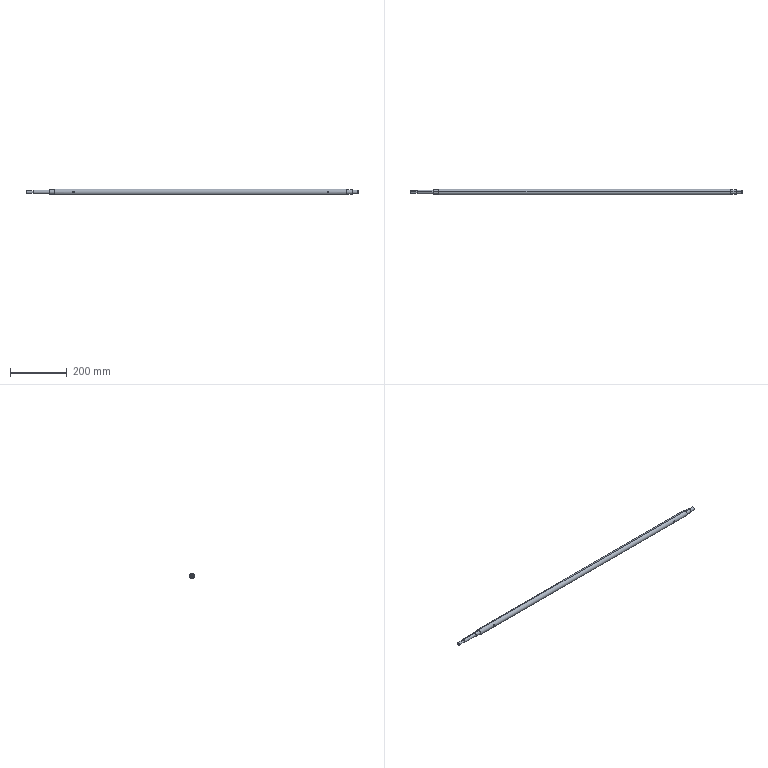Part | NX | features BREP 1 | 1 solid | 32 faces | box 1167 x 20 x 20 mm | volume 338692 mm3 | cylinder 18 | plane 10 | cone 4 | commonest cylinder face diameters 6 x4 12 x4 15 x4 4 x2 10 x2 20 x2
STEP:
#1=CARTESIAN_POINT('',(616.967,-9.539,-3.));
#2=VERTEX_POINT('',#1);
#3=CARTESIAN_POINT('',(616.967,-9.539,3.));
#4=VERTEX_POINT('',#3);
#5=CARTESIAN_POINT('',(616.967,-9.539,-3.));
#6=CARTESIAN_POINT('',(616.17,-9.539,-3.));
#7=CARTESIAN_POINT('',(614.623,-9.775,-2.35));
#8=CARTESIAN_POINT('',(613.639,-10.112,-0.004774));
#9=CARTESIAN_POINT('',(614.622,-9.775,2.351));
#10=CARTESIAN_POINT('',(616.17,-9.539,3.));
#11=CARTESIAN_POINT('',(616.967,-9.539,3.));
#12=B_SPLINE_CURVE_WITH_KNOTS('',3,(#5,#6,#7,#8,#9,#10,#11),.UNSPECIFIED.,.F.,.F.,(4,1,1,1,4),(0.,0.002358,0.004715,0.007073,0.009431),.UNSPECIFIED.);
#13=EDGE_CURVE('',#2,#4,#12,.T.);
#14=ORIENTED_EDGE('',*,*,#13,.F.);
#15=CARTESIAN_POINT('',(616.967,9.539,-3.));
#16=VERTEX_POINT('',#15);
#17=CARTESIAN_POINT('',(616.967,-10.,-3.));
#18=DIRECTION('',(0.,1.,0.));
#19=VECTOR('',#18,1000.);
#20=LINE('',#17,#19);
#21=EDGE_CURVE('',#2,#16,#20,.T.);
#22=ORIENTED_EDGE('',*,*,#21,.T.);
#23=CARTESIAN_POINT('',(616.967,9.539,3.));
#24=VERTEX_POINT('',#23);
#25=CARTESIAN_POINT('',(616.967,9.539,3.));
#26=CARTESIAN_POINT('',(616.17,9.539,3.));
#27=CARTESIAN_POINT('',(614.623,9.775,2.35));
#28=CARTESIAN_POINT('',(613.639,10.112,0.004774));
#29=CARTESIAN_POINT('',(614.622,9.775,-2.351));
#30=CARTESIAN_POINT('',(616.17,9.539,-3.));
#31=CARTESIAN_POINT('',(616.967,9.539,-3.));
#32=B_SPLINE_CURVE_WITH_KNOTS('',3,(#25,#26,#27,#28,#29,#30,#31),.UNSPECIFIED.,.F.,.F.,(4,1,1,1,4),(0.,0.002358,0.004715,0.007073,0.009431),.UNSPECIFIED.);
#33=EDGE_CURVE('',#24,#16,#32,.T.);
#34=ORIENTED_EDGE('',*,*,#33,.F.);
#35=CARTESIAN_POINT('',(616.967,-10.,3.));
#36=DIRECTION('',(0.,1.,0.));
#37=VECTOR('',#36,1000.);
#38=LINE('',#35,#37);
#39=EDGE_CURVE('',#4,#24,#38,.T.);
#40=ORIENTED_EDGE('',*,*,#39,.F.);
#41=EDGE_LOOP('',(#14,#22,#34,#40));
#42=FACE_BOUND('',#41,.T.);
#43=CARTESIAN_POINT('',(616.967,-10.,0.));
#44=DIRECTION('',(0.,1.,0.));
#45=DIRECTION('',(0.,0.,-1.));
#46=AXIS2_PLACEMENT_3D('',#43,#44,#45);
#47=CYLINDRICAL_SURFACE('',#46,3.);
#48=ADVANCED_FACE('',(#42),#47,.F.);
#49=CARTESIAN_POINT('',(-279.033,-9.539,-3.));
#50=VERTEX_POINT('',#49);
#51=CARTESIAN_POINT('',(-279.033,-9.539,3.));
#52=VERTEX_POINT('',#51);
#53=CARTESIAN_POINT('',(-279.033,-9.539,-3.));
#54=CARTESIAN_POINT('',(-279.83,-9.539,-3.));
#55=CARTESIAN_POINT('',(-281.377,-9.775,-2.35));
#56=CARTESIAN_POINT('',(-282.361,-10.112,-0.004774));
#57=CARTESIAN_POINT('',(-281.378,-9.775,2.351));
#58=CARTESIAN_POINT('',(-279.83,-9.539,3.));
#59=CARTESIAN_POINT('',(-279.033,-9.539,3.));
#60=B_SPLINE_CURVE_WITH_KNOTS('',3,(#53,#54,#55,#56,#57,#58,#59),.UNSPECIFIED.,.F.,.F.,(4,1,1,1,4),(0.,0.002358,0.004715,0.007073,0.009431),.UNSPECIFIED.);
#61=EDGE_CURVE('',#50,#52,#60,.T.);
#62=ORIENTED_EDGE('',*,*,#61,.F.);
#63=CARTESIAN_POINT('',(-279.033,9.539,-3.));
#64=VERTEX_POINT('',#63);
#65=CARTESIAN_POINT('',(-279.033,-10.,-3.));
#66=DIRECTION('',(0.,1.,0.));
#67=VECTOR('',#66,1000.);
#68=LINE('',#65,#67);
#69=EDGE_CURVE('',#50,#64,#68,.T.);
#70=ORIENTED_EDGE('',*,*,#69,.T.);
#71=CARTESIAN_POINT('',(-279.033,9.539,3.));
#72=VERTEX_POINT('',#71);
#73=CARTESIAN_POINT('',(-279.033,9.539,3.));
#74=CARTESIAN_POINT('',(-279.83,9.539,3.));
#75=CARTESIAN_POINT('',(-281.377,9.775,2.35));
#76=CARTESIAN_POINT('',(-282.361,10.112,0.004774));
#77=CARTESIAN_POINT('',(-281.378,9.775,-2.351));
#78=CARTESIAN_POINT('',(-279.83,9.539,-3.));
#79=CARTESIAN_POINT('',(-279.033,9.539,-3.));
#80=B_SPLINE_CURVE_WITH_KNOTS('',3,(#73,#74,#75,#76,#77,#78,#79),.UNSPECIFIED.,.F.,.F.,(4,1,1,1,4),(0.,0.002358,0.004715,0.007073,0.009431),.UNSPECIFIED.);
#81=EDGE_CURVE('',#72,#64,#80,.T.);
#82=ORIENTED_EDGE('',*,*,#81,.F.);
#83=CARTESIAN_POINT('',(-279.033,-10.,3.));
#84=DIRECTION('',(0.,1.,0.));
#85=VECTOR('',#84,1000.);
#86=LINE('',#83,#85);
#87=EDGE_CURVE('',#52,#72,#86,.T.);
#88=ORIENTED_EDGE('',*,*,#87,.F.);
#89=EDGE_LOOP('',(#62,#70,#82,#88));
#90=FACE_BOUND('',#89,.T.);
#91=CARTESIAN_POINT('',(-279.033,-10.,0.));
#92=DIRECTION('',(0.,1.,0.));
#93=DIRECTION('',(0.,0.,-1.));
#94=AXIS2_PLACEMENT_3D('',#91,#92,#93);
#95=CYLINDRICAL_SURFACE('',#94,3.);
#96=ADVANCED_FACE('',(#90),#95,.F.);
#97=CARTESIAN_POINT('',(721.967,0.,5.));
#98=VERTEX_POINT('',#97);
#99=CARTESIAN_POINT('',(721.967,0.,-5.));
#100=VERTEX_POINT('',#99);
#101=CARTESIAN_POINT('',(721.967,0.,0.));
#102=DIRECTION('',(-1.,0.,0.));
#103=DIRECTION('',(0.,0.,1.));
#104=AXIS2_PLACEMENT_3D('',#101,#102,#103);
#105=CIRCLE('',#104,5.);
#106=EDGE_CURVE('',#98,#100,#105,.T.);
#107=ORIENTED_EDGE('',*,*,#106,.T.);
#108=CARTESIAN_POINT('',(720.967,0.,-6.));
#109=VERTEX_POINT('',#108);
#110=CARTESIAN_POINT('',(721.967,0.,-5.));
#111=DIRECTION('',(-0.7071,0.,-0.7071));
#112=VECTOR('',#111,1000.);
#113=LINE('',#110,#112);
#114=EDGE_CURVE('',#100,#109,#113,.T.);
#115=ORIENTED_EDGE('',*,*,#114,.T.);
#116=CARTESIAN_POINT('',(720.967,0.,6.));
#117=VERTEX_POINT('',#116);
#118=CARTESIAN_POINT('',(720.967,0.,0.));
#119=DIRECTION('',(-1.,0.,0.));
#120=DIRECTION('',(0.,0.,1.));
#121=AXIS2_PLACEMENT_3D('',#118,#119,#120);
#122=CIRCLE('',#121,6.);
#123=EDGE_CURVE('',#117,#109,#122,.T.);
#124=ORIENTED_EDGE('',*,*,#123,.F.);
#125=CARTESIAN_POINT('',(721.967,0.,5.));
#126=DIRECTION('',(-0.7071,0.,0.7071));
#127=VECTOR('',#126,1000.);
#128=LINE('',#125,#127);
#129=EDGE_CURVE('',#98,#117,#128,.T.);
#130=ORIENTED_EDGE('',*,*,#129,.F.);
#131=EDGE_LOOP('',(#107,#115,#124,#130));
#132=FACE_BOUND('',#131,.T.);
#133=CARTESIAN_POINT('',(721.967,0.,0.));
#134=DIRECTION('',(-1.,0.,0.));
#135=DIRECTION('',(0.,0.,-1.));
#136=AXIS2_PLACEMENT_3D('',#133,#134,#135);
#137=CONICAL_SURFACE('',#136,5.,0.7854);
#138=ADVANCED_FACE('',(#132),#137,.T.);
#139=ORIENTED_EDGE('',*,*,#123,.T.);
#140=CARTESIAN_POINT('',(701.967,0.,-6.));
#141=VERTEX_POINT('',#140);
#142=CARTESIAN_POINT('',(-445.033,0.,-6.));
#143=DIRECTION('',(-1.,0.,0.));
#144=VECTOR('',#143,1000.);
#145=LINE('',#142,#144);
#146=EDGE_CURVE('',#109,#141,#145,.T.);
#147=ORIENTED_EDGE('',*,*,#146,.T.);
#148=CARTESIAN_POINT('',(701.967,0.,6.));
#149=VERTEX_POINT('',#148);
#150=CARTESIAN_POINT('',(701.967,0.,0.));
#151=DIRECTION('',(-1.,0.,0.));
#152=DIRECTION('',(0.,0.,1.));
#153=AXIS2_PLACEMENT_3D('',#150,#151,#152);
#154=CIRCLE('',#153,6.);
#155=EDGE_CURVE('',#149,#141,#154,.T.);
#156=ORIENTED_EDGE('',*,*,#155,.F.);
#157=CARTESIAN_POINT('',(-445.033,0.,6.));
#158=DIRECTION('',(-1.,0.,0.));
#159=VECTOR('',#158,1000.);
#160=LINE('',#157,#159);
#161=EDGE_CURVE('',#117,#149,#160,.T.);
#162=ORIENTED_EDGE('',*,*,#161,.F.);
#163=EDGE_LOOP('',(#139,#147,#156,#162));
#164=FACE_BOUND('',#163,.T.);
#165=CARTESIAN_POINT('',(-445.033,0.,0.));
#166=DIRECTION('',(-1.,0.,0.));
#167=DIRECTION('',(0.,0.,-1.));
#168=AXIS2_PLACEMENT_3D('',#165,#166,#167);
#169=CYLINDRICAL_SURFACE('',#168,6.);
#170=ADVANCED_FACE('',(#164),#169,.T.);
#171=CARTESIAN_POINT('',(701.967,0.,7.5));
#172=VERTEX_POINT('',#171);
#173=CARTESIAN_POINT('',(701.967,0.,-7.5));
#174=VERTEX_POINT('',#173);
#175=CARTESIAN_POINT('',(701.967,0.,0.));
#176=DIRECTION('',(-1.,0.,0.));
#177=DIRECTION('',(0.,0.,1.));
#178=AXIS2_PLACEMENT_3D('',#175,#176,#177);
#179=CIRCLE('',#178,7.5);
#180=EDGE_CURVE('',#172,#174,#179,.T.);
#181=ORIENTED_EDGE('',*,*,#180,.T.);
#182=CARTESIAN_POINT('',(681.967,0.,-7.5));
#183=VERTEX_POINT('',#182);
#184=CARTESIAN_POINT('',(-445.033,0.,-7.5));
#185=DIRECTION('',(-1.,0.,0.));
#186=VECTOR('',#185,1000.);
#187=LINE('',#184,#186);
#188=EDGE_CURVE('',#174,#183,#187,.T.);
#189=ORIENTED_EDGE('',*,*,#188,.T.);
#190=CARTESIAN_POINT('',(681.967,0.,7.5));
#191=VERTEX_POINT('',#190);
#192=CARTESIAN_POINT('',(681.967,0.,0.));
#193=DIRECTION('',(-1.,0.,0.));
#194=DIRECTION('',(0.,0.,1.));
#195=AXIS2_PLACEMENT_3D('',#192,#193,#194);
#196=CIRCLE('',#195,7.5);
#197=EDGE_CURVE('',#191,#183,#196,.T.);
#198=ORIENTED_EDGE('',*,*,#197,.F.);
#199=CARTESIAN_POINT('',(-445.033,0.,7.5));
#200=DIRECTION('',(-1.,0.,0.));
#201=VECTOR('',#200,1000.);
#202=LINE('',#199,#201);
#203=EDGE_CURVE('',#172,#191,#202,.T.);
#204=ORIENTED_EDGE('',*,*,#203,.F.);
#205=EDGE_LOOP('',(#181,#189,#198,#204));
#206=FACE_BOUND('',#205,.T.);
#207=CARTESIAN_POINT('',(-445.033,0.,0.));
#208=DIRECTION('',(-1.,0.,0.));
#209=DIRECTION('',(0.,0.,-1.));
#210=AXIS2_PLACEMENT_3D('',#207,#208,#209);
#211=CYLINDRICAL_SURFACE('',#210,7.5);
#212=ADVANCED_FACE('',(#206),#211,.T.);
#213=CARTESIAN_POINT('',(681.967,0.,10.));
#214=VERTEX_POINT('',#213);
#215=CARTESIAN_POINT('',(681.967,0.,-10.));
#216=VERTEX_POINT('',#215);
#217=CARTESIAN_POINT('',(681.967,0.,0.));
#218=DIRECTION('',(-1.,0.,0.));
#219=DIRECTION('',(0.,0.,1.));
#220=AXIS2_PLACEMENT_3D('',#217,#218,#219);
#221=CIRCLE('',#220,10.);
#222=EDGE_CURVE('',#214,#216,#221,.T.);
#223=ORIENTED_EDGE('',*,*,#222,.T.);
#224=CARTESIAN_POINT('',(-344.033,0.,-10.));
#225=VERTEX_POINT('',#224);
#226=CARTESIAN_POINT('',(-445.033,0.,-10.));
#227=DIRECTION('',(-1.,0.,0.));
#228=VECTOR('',#227,1000.);
#229=LINE('',#226,#228);
#230=EDGE_CURVE('',#216,#225,#229,.T.);
#231=ORIENTED_EDGE('',*,*,#230,.T.);
#232=CARTESIAN_POINT('',(-344.033,0.,10.));
#233=VERTEX_POINT('',#232);
#234=CARTESIAN_POINT('',(-344.033,0.,0.));
#235=DIRECTION('',(-1.,0.,0.));
#236=DIRECTION('',(0.,0.,1.));
#237=AXIS2_PLACEMENT_3D('',#234,#235,#236);
#238=CIRCLE('',#237,10.);
#239=EDGE_CURVE('',#233,#225,#238,.T.);
#240=ORIENTED_EDGE('',*,*,#239,.F.);
#241=CARTESIAN_POINT('',(-445.033,0.,10.));
#242=DIRECTION('',(-1.,0.,0.));
#243=VECTOR('',#242,1000.);
#244=LINE('',#241,#243);
#245=EDGE_CURVE('',#214,#233,#244,.T.);
#246=ORIENTED_EDGE('',*,*,#245,.F.);
#247=EDGE_LOOP('',(#223,#231,#240,#246));
#248=FACE_BOUND('',#247,.T.);
#249=ORIENTED_EDGE('',*,*,#81,.T.);
#250=CARTESIAN_POINT('',(-279.033,9.539,-3.));
#251=CARTESIAN_POINT('',(-278.235,9.539,-3.));
#252=CARTESIAN_POINT('',(-276.689,9.775,-2.35));
#253=CARTESIAN_POINT('',(-275.705,10.112,-0.004774));
#254=CARTESIAN_POINT('',(-276.688,9.775,2.351));
#255=CARTESIAN_POINT('',(-278.235,9.539,3.));
#256=CARTESIAN_POINT('',(-279.033,9.539,3.));
#257=B_SPLINE_CURVE_WITH_KNOTS('',3,(#250,#251,#252,#253,#254,#255,#256),.UNSPECIFIED.,.F.,.F.,(4,1,1,1,4),(0.,0.002358,0.004715,0.007073,0.009431),.UNSPECIFIED.);
#258=EDGE_CURVE('',#64,#72,#257,.T.);
#259=ORIENTED_EDGE('',*,*,#258,.T.);
#260=EDGE_LOOP('',(#249,#259));
#261=FACE_BOUND('',#260,.T.);
#262=ORIENTED_EDGE('',*,*,#33,.T.);
#263=CARTESIAN_POINT('',(616.967,9.539,-3.));
#264=CARTESIAN_POINT('',(617.765,9.539,-3.));
#265=CARTESIAN_POINT('',(619.311,9.775,-2.35));
#266=CARTESIAN_POINT('',(620.295,10.112,-0.004774));
#267=CARTESIAN_POINT('',(619.312,9.775,2.351));
#268=CARTESIAN_POINT('',(617.765,9.539,3.));
#269=CARTESIAN_POINT('',(616.967,9.539,3.));
#270=B_SPLINE_CURVE_WITH_KNOTS('',3,(#263,#264,#265,#266,#267,#268,#269),.UNSPECIFIED.,.F.,.F.,(4,1,1,1,4),(0.,0.002358,0.004715,0.007073,0.009431),.UNSPECIFIED.);
#271=EDGE_CURVE('',#16,#24,#270,.T.);
#272=ORIENTED_EDGE('',*,*,#271,.T.);
#273=EDGE_LOOP('',(#262,#272));
#274=FACE_BOUND('',#273,.T.);
#275=CARTESIAN_POINT('',(-445.033,0.,0.));
#276=DIRECTION('',(-1.,0.,0.));
#277=DIRECTION('',(0.,0.,-1.));
#278=AXIS2_PLACEMENT_3D('',#275,#276,#277);
#279=CYLINDRICAL_SURFACE('',#278,10.);
#280=ADVANCED_FACE('',(#248,#261,#274),#279,.T.);
#281=CARTESIAN_POINT('',(-344.033,0.,7.5));
#282=VERTEX_POINT('',#281);
#283=CARTESIAN_POINT('',(-344.033,0.,-7.5));
#284=VERTEX_POINT('',#283);
#285=CARTESIAN_POINT('',(-344.033,0.,0.));
#286=DIRECTION('',(-1.,0.,0.));
#287=DIRECTION('',(0.,0.,1.));
#288=AXIS2_PLACEMENT_3D('',#285,#286,#287);
#289=CIRCLE('',#288,7.5);
#290=EDGE_CURVE('',#282,#284,#289,.T.);
#291=ORIENTED_EDGE('',*,*,#290,.T.);
#292=CARTESIAN_POINT('',(-364.033,0.,-7.5));
#293=VERTEX_POINT('',#292);
#294=CARTESIAN_POINT('',(-445.033,0.,-7.5));
#295=DIRECTION('',(-1.,0.,0.));
#296=VECTOR('',#295,1000.);
#297=LINE('',#294,#296);
#298=EDGE_CURVE('',#284,#293,#297,.T.);
#299=ORIENTED_EDGE('',*,*,#298,.T.);
#300=CARTESIAN_POINT('',(-364.033,0.,7.5));
#301=VERTEX_POINT('',#300);
#302=CARTESIAN_POINT('',(-364.033,0.,0.));
#303=DIRECTION('',(-1.,0.,0.));
#304=DIRECTION('',(0.,0.,1.));
#305=AXIS2_PLACEMENT_3D('',#302,#303,#304);
#306=CIRCLE('',#305,7.5);
#307=EDGE_CURVE('',#301,#293,#306,.T.);
#308=ORIENTED_EDGE('',*,*,#307,.F.);
#309=CARTESIAN_POINT('',(-445.033,0.,7.5));
#310=DIRECTION('',(-1.,0.,0.));
#311=VECTOR('',#310,1000.);
#312=LINE('',#309,#311);
#313=EDGE_CURVE('',#282,#301,#312,.T.);
#314=ORIENTED_EDGE('',*,*,#313,.F.);
#315=EDGE_LOOP('',(#291,#299,#308,#314));
#316=FACE_BOUND('',#315,.T.);
#317=CARTESIAN_POINT('',(-445.033,0.,0.));
#318=DIRECTION('',(-1.,0.,0.));
#319=DIRECTION('',(0.,0.,-1.));
#320=AXIS2_PLACEMENT_3D('',#317,#318,#319);
#321=CYLINDRICAL_SURFACE('',#320,7.5);
#322=ADVANCED_FACE('',(#316),#321,.T.);
#323=CARTESIAN_POINT('',(-364.033,0.,6.));
#324=VERTEX_POINT('',#323);
#325=CARTESIAN_POINT('',(-364.033,0.,-6.));
#326=VERTEX_POINT('',#325);
#327=CARTESIAN_POINT('',(-364.033,0.,0.));
#328=DIRECTION('',(-1.,0.,0.));
#329=DIRECTION('',(0.,0.,1.));
#330=AXIS2_PLACEMENT_3D('',#327,#328,#329);
#331=CIRCLE('',#330,6.);
#332=EDGE_CURVE('',#324,#326,#331,.T.);
#333=ORIENTED_EDGE('',*,*,#332,.T.);
#334=CARTESIAN_POINT('',(-420.033,0.,-6.));
#335=VERTEX_POINT('',#334);
#336=CARTESIAN_POINT('',(-445.033,0.,-6.));
#337=DIRECTION('',(-1.,0.,0.));
#338=VECTOR('',#337,1000.);
#339=LINE('',#336,#338);
#340=EDGE_CURVE('',#326,#335,#339,.T.);
#341=ORIENTED_EDGE('',*,*,#340,.T.);
#342=CARTESIAN_POINT('',(-420.033,0.,6.));
#343=VERTEX_POINT('',#342);
#344=CARTESIAN_POINT('',(-420.033,0.,0.));
#345=DIRECTION('',(-1.,0.,0.));
#346=DIRECTION('',(0.,0.,1.));
#347=AXIS2_PLACEMENT_3D('',#344,#345,#346);
#348=CIRCLE('',#347,6.);
#349=EDGE_CURVE('',#343,#335,#348,.T.);
#350=ORIENTED_EDGE('',*,*,#349,.F.);
#351=CARTESIAN_POINT('',(-445.033,0.,6.));
#352=DIRECTION('',(-1.,0.,0.));
#353=VECTOR('',#352,1000.);
#354=LINE('',#351,#353);
#355=EDGE_CURVE('',#324,#343,#354,.T.);
#356=ORIENTED_EDGE('',*,*,#355,.F.);
#357=EDGE_LOOP('',(#333,#341,#350,#356));
#358=FACE_BOUND('',#357,.T.);
#359=CARTESIAN_POINT('',(-445.033,0.,0.));
#360=DIRECTION('',(-1.,0.,0.));
#361=DIRECTION('',(0.,0.,-1.));
#362=AXIS2_PLACEMENT_3D('',#359,#360,#361);
#363=CYLINDRICAL_SURFACE('',#362,6.);
#364=ADVANCED_FACE('',(#358),#363,.T.);
#365=CARTESIAN_POINT('',(-420.033,0.,5.));
#366=VERTEX_POINT('',#365);
#367=CARTESIAN_POINT('',(-420.033,0.,-5.));
#368=VERTEX_POINT('',#367);
#369=CARTESIAN_POINT('',(-420.033,0.,0.));
#370=DIRECTION('',(-1.,0.,0.));
#371=DIRECTION('',(0.,0.,1.));
#372=AXIS2_PLACEMENT_3D('',#369,#370,#371);
#373=CIRCLE('',#372,5.);
#374=EDGE_CURVE('',#366,#368,#373,.T.);
#375=ORIENTED_EDGE('',*,*,#374,.T.);
#376=CARTESIAN_POINT('',(-444.033,0.,-5.));
#377=VERTEX_POINT('',#376);
#378=CARTESIAN_POINT('',(-445.033,0.,-5.));
#379=DIRECTION('',(-1.,0.,0.));
#380=VECTOR('',#379,1000.);
#381=LINE('',#378,#380);
#382=EDGE_CURVE('',#368,#377,#381,.T.);
#383=ORIENTED_EDGE('',*,*,#382,.T.);
#384=CARTESIAN_POINT('',(-444.033,0.,5.));
#385=VERTEX_POINT('',#384);
#386=CARTESIAN_POINT('',(-444.033,0.,0.));
#387=DIRECTION('',(-1.,0.,0.));
#388=DIRECTION('',(0.,0.,1.));
#389=AXIS2_PLACEMENT_3D('',#386,#387,#388);
#390=CIRCLE('',#389,5.);
#391=EDGE_CURVE('',#385,#377,#390,.T.);
#392=ORIENTED_EDGE('',*,*,#391,.F.);
#393=CARTESIAN_POINT('',(-445.033,0.,5.));
#394=DIRECTION('',(-1.,0.,0.));
#395=VECTOR('',#394,1000.);
#396=LINE('',#393,#395);
#397=EDGE_CURVE('',#366,#385,#396,.T.);
#398=ORIENTED_EDGE('',*,*,#397,.F.);
#399=EDGE_LOOP('',(#375,#383,#392,#398));
#400=FACE_BOUND('',#399,.T.);
#401=CARTESIAN_POINT('',(-437.033,4.583,-2.));
#402=VERTEX_POINT('',#401);
#403=CARTESIAN_POINT('',(-425.033,4.583,-2.));
#404=VERTEX_POINT('',#403);
#405=CARTESIAN_POINT('',(-445.033,4.583,-2.));
#406=DIRECTION('',(1.,0.,0.));
#407=VECTOR('',#406,1000.);
#408=LINE('',#405,#407);
#409=EDGE_CURVE('',#402,#404,#408,.T.);
#410=ORIENTED_EDGE('',*,*,#409,.T.);
#411=CARTESIAN_POINT('',(-425.033,4.583,2.));
#412=VERTEX_POINT('',#411);
#413=CARTESIAN_POINT('',(-425.033,4.583,-2.));
#414=CARTESIAN_POINT('',(-424.498,4.583,-2.));
#415=CARTESIAN_POINT('',(-423.472,4.8,-1.567));
#416=CARTESIAN_POINT('',(-422.813,5.1,-0.004067));
#417=CARTESIAN_POINT('',(-423.472,4.8,1.568));
#418=CARTESIAN_POINT('',(-424.498,4.583,2.));
#419=CARTESIAN_POINT('',(-425.033,4.583,2.));
#420=B_SPLINE_CURVE_WITH_KNOTS('',3,(#413,#414,#415,#416,#417,#418,#419),.UNSPECIFIED.,.F.,.F.,(4,1,1,1,4),(0.,0.001579,0.003158,0.004737,0.006317),.UNSPECIFIED.);
#421=EDGE_CURVE('',#404,#412,#420,.T.);
#422=ORIENTED_EDGE('',*,*,#421,.T.);
#423=CARTESIAN_POINT('',(-437.033,4.583,2.));
#424=VERTEX_POINT('',#423);
#425=CARTESIAN_POINT('',(-445.033,4.583,2.));
#426=DIRECTION('',(-1.,0.,0.));
#427=VECTOR('',#426,1000.);
#428=LINE('',#425,#427);
#429=EDGE_CURVE('',#412,#424,#428,.T.);
#430=ORIENTED_EDGE('',*,*,#429,.T.);
#431=CARTESIAN_POINT('',(-437.033,4.583,2.));
#432=CARTESIAN_POINT('',(-437.567,4.583,2.));
#433=CARTESIAN_POINT('',(-438.593,4.8,1.567));
#434=CARTESIAN_POINT('',(-439.252,5.1,0.004067));
#435=CARTESIAN_POINT('',(-438.594,4.8,-1.568));
#436=CARTESIAN_POINT('',(-437.567,4.583,-2.));
#437=CARTESIAN_POINT('',(-437.033,4.583,-2.));
#438=B_SPLINE_CURVE_WITH_KNOTS('',3,(#431,#432,#433,#434,#435,#436,#437),.UNSPECIFIED.,.F.,.F.,(4,1,1,1,4),(0.,0.001579,0.003158,0.004737,0.006317),.UNSPECIFIED.);
#439=EDGE_CURVE('',#424,#402,#438,.T.);
#440=ORIENTED_EDGE('',*,*,#439,.T.);
#441=EDGE_LOOP('',(#410,#422,#430,#440));
#442=FACE_BOUND('',#441,.T.);
#443=CARTESIAN_POINT('',(-445.033,0.,0.));
#444=DIRECTION('',(-1.,0.,0.));
#445=DIRECTION('',(0.,0.,-1.));
#446=AXIS2_PLACEMENT_3D('',#443,#444,#445);
#447=CYLINDRICAL_SURFACE('',#446,5.);
#448=ADVANCED_FACE('',(#400,#442),#447,.T.);
#449=CARTESIAN_POINT('',(-445.033,0.,4.));
#450=VERTEX_POINT('',#449);
#451=CARTESIAN_POINT('',(-445.033,0.,-4.));
#452=VERTEX_POINT('',#451);
#453=CARTESIAN_POINT('',(-445.033,0.,0.));
#454=DIRECTION('',(-1.,0.,0.));
#455=DIRECTION('',(0.,0.,1.));
#456=AXIS2_PLACEMENT_3D('',#453,#454,#455);
#457=CIRCLE('',#456,4.);
#458=EDGE_CURVE('',#450,#452,#457,.T.);
#459=ORIENTED_EDGE('',*,*,#458,.F.);
#460=CARTESIAN_POINT('',(-444.033,0.,5.));
#461=DIRECTION('',(0.7071,0.,0.7071));
#462=VECTOR('',#461,1000.);
#463=LINE('',#460,#462);
#464=EDGE_CURVE('',#385,#450,#463,.F.);
#465=ORIENTED_EDGE('',*,*,#464,.F.);
#466=ORIENTED_EDGE('',*,*,#391,.T.);
#467=CARTESIAN_POINT('',(-444.033,0.,-5.));
#468=DIRECTION('',(0.7071,0.,-0.7071));
#469=VECTOR('',#468,1000.);
#470=LINE('',#467,#469);
#471=EDGE_CURVE('',#377,#452,#470,.F.);
#472=ORIENTED_EDGE('',*,*,#471,.T.);
#473=EDGE_LOOP('',(#459,#465,#466,#472));
#474=FACE_BOUND('',#473,.T.);
#475=CARTESIAN_POINT('',(-444.033,0.,0.));
#476=DIRECTION('',(1.,0.,0.));
#477=DIRECTION('',(0.,0.,1.));
#478=AXIS2_PLACEMENT_3D('',#475,#476,#477);
#479=CONICAL_SURFACE('',#478,5.,0.7854);
#480=ADVANCED_FACE('',(#474),#479,.T.);
#481=ORIENTED_EDGE('',*,*,#464,.T.);
#482=CARTESIAN_POINT('',(-445.033,0.,0.));
#483=DIRECTION('',(-1.,0.,0.));
#484=DIRECTION('',(0.,0.,1.));
#485=AXIS2_PLACEMENT_3D('',#482,#483,#484);
#486=CIRCLE('',#485,4.);
#487=EDGE_CURVE('',#452,#450,#486,.T.);
#488=ORIENTED_EDGE('',*,*,#487,.F.);
#489=ORIENTED_EDGE('',*,*,#471,.F.);
#490=CARTESIAN_POINT('',(-444.033,0.,0.));
#491=DIRECTION('',(-1.,0.,0.));
#492=DIRECTION('',(0.,0.,1.));
#493=AXIS2_PLACEMENT_3D('',#490,#491,#492);
#494=CIRCLE('',#493,5.);
#495=EDGE_CURVE('',#377,#385,#494,.T.);
#496=ORIENTED_EDGE('',*,*,#495,.T.);
#497=EDGE_LOOP('',(#481,#488,#489,#496));
#498=FACE_BOUND('',#497,.T.);
#499=CARTESIAN_POINT('',(-444.033,0.,0.));
#500=DIRECTION('',(1.,0.,0.));
#501=DIRECTION('',(0.,0.,1.));
#502=AXIS2_PLACEMENT_3D('',#499,#500,#501);
#503=CONICAL_SURFACE('',#502,5.,0.7854);
#504=ADVANCED_FACE('',(#498),#503,.T.);
#505=ORIENTED_EDGE('',*,*,#382,.F.);
#506=CARTESIAN_POINT('',(-420.033,0.,0.));
#507=DIRECTION('',(-1.,0.,0.));
#508=DIRECTION('',(0.,0.,1.));
#509=AXIS2_PLACEMENT_3D('',#506,#507,#508);
#510=CIRCLE('',#509,5.);
#511=EDGE_CURVE('',#368,#366,#510,.T.);
#512=ORIENTED_EDGE('',*,*,#511,.T.);
#513=ORIENTED_EDGE('',*,*,#397,.T.);
#514=ORIENTED_EDGE('',*,*,#495,.F.);
#515=EDGE_LOOP('',(#505,#512,#513,#514));
#516=FACE_BOUND('',#515,.T.);
#517=CARTESIAN_POINT('',(-445.033,0.,0.));
#518=DIRECTION('',(-1.,0.,0.));
#519=DIRECTION('',(0.,0.,-1.));
#520=AXIS2_PLACEMENT_3D('',#517,#518,#519);
#521=CYLINDRICAL_SURFACE('',#520,5.);
#522=ADVANCED_FACE('',(#516),#521,.T.);
#523=ORIENTED_EDGE('',*,*,#349,.T.);
#524=CARTESIAN_POINT('',(-420.033,0.,0.));
#525=DIRECTION('',(-1.,0.,0.));
#526=DIRECTION('',(0.,0.,1.));
#527=AXIS2_PLACEMENT_3D('',#524,#525,#526);
#528=CIRCLE('',#527,6.);
#529=EDGE_CURVE('',#335,#343,#528,.T.);
#530=ORIENTED_EDGE('',*,*,#529,.T.);
#531=EDGE_LOOP('',(#523,#530));
#532=FACE_BOUND('',#531,.T.);
#533=ORIENTED_EDGE('',*,*,#374,.F.);
#534=ORIENTED_EDGE('',*,*,#511,.F.);
#535=EDGE_LOOP('',(#533,#534));
#536=FACE_BOUND('',#535,.T.);
#537=CARTESIAN_POINT('',(-420.033,5.,0.));
#538=DIRECTION('',(1.,0.,0.));
#539=DIRECTION('',(0.,0.,1.));
#540=AXIS2_PLACEMENT_3D('',#537,#538,#539);
#541=PLANE('',#540);
#542=ADVANCED_FACE('',(#532,#536),#541,.F.);
#543=ORIENTED_EDGE('',*,*,#340,.F.);
#544=CARTESIAN_POINT('',(-364.033,0.,0.));
#545=DIRECTION('',(-1.,0.,0.));
#546=DIRECTION('',(0.,0.,1.));
#547=AXIS2_PLACEMENT_3D('',#544,#545,#546);
#548=CIRCLE('',#547,6.);
#549=EDGE_CURVE('',#326,#324,#548,.T.);
#550=ORIENTED_EDGE('',*,*,#549,.T.);
#551=ORIENTED_EDGE('',*,*,#355,.T.);
#552=ORIENTED_EDGE('',*,*,#529,.F.);
#553=EDGE_LOOP('',(#543,#550,#551,#552));
#554=FACE_BOUND('',#553,.T.);
#555=CARTESIAN_POINT('',(-445.033,0.,0.));
#556=DIRECTION('',(-1.,0.,0.));
#557=DIRECTION('',(0.,0.,-1.));
#558=AXIS2_PLACEMENT_3D('',#555,#556,#557);
#559=CYLINDRICAL_SURFACE('',#558,6.);
#560=ADVANCED_FACE('',(#554),#559,.T.);
#561=ORIENTED_EDGE('',*,*,#307,.T.);
#562=CARTESIAN_POINT('',(-364.033,0.,0.));
#563=DIRECTION('',(-1.,0.,0.));
#564=DIRECTION('',(0.,0.,1.));
#565=AXIS2_PLACEMENT_3D('',#562,#563,#564);
#566=CIRCLE('',#565,7.5);
#567=EDGE_CURVE('',#293,#301,#566,.T.);
#568=ORIENTED_EDGE('',*,*,#567,.T.);
#569=EDGE_LOOP('',(#561,#568));
#570=FACE_BOUND('',#569,.T.);
#571=ORIENTED_EDGE('',*,*,#332,.F.);
#572=ORIENTED_EDGE('',*,*,#549,.F.);
#573=EDGE_LOOP('',(#571,#572));
#574=FACE_BOUND('',#573,.T.);
#575=CARTESIAN_POINT('',(-364.033,6.,0.));
#576=DIRECTION('',(1.,0.,0.));
#577=DIRECTION('',(0.,0.,1.));
#578=AXIS2_PLACEMENT_3D('',#575,#576,#577);
#579=PLANE('',#578);
#580=ADVANCED_FACE('',(#570,#574),#579,.F.);
#581=ORIENTED_EDGE('',*,*,#298,.F.);
#582=CARTESIAN_POINT('',(-344.033,0.,0.));
#583=DIRECTION('',(-1.,0.,0.));
#584=DIRECTION('',(0.,0.,1.));
#585=AXIS2_PLACEMENT_3D('',#582,#583,#584);
#586=CIRCLE('',#585,7.5);
#587=EDGE_CURVE('',#284,#282,#586,.T.);
#588=ORIENTED_EDGE('',*,*,#587,.T.);
#589=ORIENTED_EDGE('',*,*,#313,.T.);
#590=ORIENTED_EDGE('',*,*,#567,.F.);
#591=EDGE_LOOP('',(#581,#588,#589,#590));
#592=FACE_BOUND('',#591,.T.);
#593=CARTESIAN_POINT('',(-445.033,0.,0.));
#594=DIRECTION('',(-1.,0.,0.));
#595=DIRECTION('',(0.,0.,-1.));
#596=AXIS2_PLACEMENT_3D('',#593,#594,#595);
#597=CYLINDRICAL_SURFACE('',#596,7.5);
#598=ADVANCED_FACE('',(#592),#597,.T.);
#599=ORIENTED_EDGE('',*,*,#239,.T.);
#600=CARTESIAN_POINT('',(-344.033,0.,0.));
#601=DIRECTION('',(-1.,0.,0.));
#602=DIRECTION('',(0.,0.,1.));
#603=AXIS2_PLACEMENT_3D('',#600,#601,#602);
#604=CIRCLE('',#603,10.);
#605=EDGE_CURVE('',#225,#233,#604,.T.);
#606=ORIENTED_EDGE('',*,*,#605,.T.);
#607=EDGE_LOOP('',(#599,#606));
#608=FACE_BOUND('',#607,.T.);
#609=ORIENTED_EDGE('',*,*,#290,.F.);
#610=ORIENTED_EDGE('',*,*,#587,.F.);
#611=EDGE_LOOP('',(#609,#610));
#612=FACE_BOUND('',#611,.T.);
#613=CARTESIAN_POINT('',(-344.033,7.5,0.));
#614=DIRECTION('',(1.,0.,0.));
#615=DIRECTION('',(0.,0.,1.));
#616=AXIS2_PLACEMENT_3D('',#613,#614,#615);
#617=PLANE('',#616);
#618=ADVANCED_FACE('',(#608,#612),#617,.F.);
#619=ORIENTED_EDGE('',*,*,#230,.F.);
#620=CARTESIAN_POINT('',(681.967,0.,0.));
#621=DIRECTION('',(-1.,0.,0.));
#622=DIRECTION('',(0.,0.,1.));
#623=AXIS2_PLACEMENT_3D('',#620,#621,#622);
#624=CIRCLE('',#623,10.);
#625=EDGE_CURVE('',#216,#214,#624,.T.);
#626=ORIENTED_EDGE('',*,*,#625,.T.);
#627=ORIENTED_EDGE('',*,*,#245,.T.);
#628=ORIENTED_EDGE('',*,*,#605,.F.);
#629=EDGE_LOOP('',(#619,#626,#627,#628));
#630=FACE_BOUND('',#629,.T.);
#631=CARTESIAN_POINT('',(616.967,-9.539,3.));
#632=CARTESIAN_POINT('',(617.765,-9.539,3.));
#633=CARTESIAN_POINT('',(619.311,-9.775,2.35));
#634=CARTESIAN_POINT('',(620.295,-10.112,0.004774));
#635=CARTESIAN_POINT('',(619.312,-9.775,-2.351));
#636=CARTESIAN_POINT('',(617.765,-9.539,-3.));
#637=CARTESIAN_POINT('',(616.967,-9.539,-3.));
#638=B_SPLINE_CURVE_WITH_KNOTS('',3,(#631,#632,#633,#634,#635,#636,#637),.UNSPECIFIED.,.F.,.F.,(4,1,1,1,4),(0.,0.002358,0.004715,0.007073,0.009431),.UNSPECIFIED.);
#639=EDGE_CURVE('',#4,#2,#638,.T.);
#640=ORIENTED_EDGE('',*,*,#639,.T.);
#641=ORIENTED_EDGE('',*,*,#13,.T.);
#642=EDGE_LOOP('',(#640,#641));
#643=FACE_BOUND('',#642,.T.);
#644=CARTESIAN_POINT('',(-279.033,-9.539,3.));
#645=CARTESIAN_POINT('',(-278.235,-9.539,3.));
#646=CARTESIAN_POINT('',(-276.689,-9.775,2.35));
#647=CARTESIAN_POINT('',(-275.705,-10.112,0.004774));
#648=CARTESIAN_POINT('',(-276.688,-9.775,-2.351));
#649=CARTESIAN_POINT('',(-278.235,-9.539,-3.));
#650=CARTESIAN_POINT('',(-279.033,-9.539,-3.));
#651=B_SPLINE_CURVE_WITH_KNOTS('',3,(#644,#645,#646,#647,#648,#649,#650),.UNSPECIFIED.,.F.,.F.,(4,1,1,1,4),(0.,0.002358,0.004715,0.007073,0.009431),.UNSPECIFIED.);
#652=EDGE_CURVE('',#52,#50,#651,.T.);
#653=ORIENTED_EDGE('',*,*,#652,.T.);
#654=ORIENTED_EDGE('',*,*,#61,.T.);
#655=EDGE_LOOP('',(#653,#654));
#656=FACE_BOUND('',#655,.T.);
#657=CARTESIAN_POINT('',(-445.033,0.,0.));
#658=DIRECTION('',(-1.,0.,0.));
#659=DIRECTION('',(0.,0.,-1.));
#660=AXIS2_PLACEMENT_3D('',#657,#658,#659);
#661=CYLINDRICAL_SURFACE('',#660,10.);
#662=ADVANCED_FACE('',(#630,#643,#656),#661,.T.);
#663=ORIENTED_EDGE('',*,*,#222,.F.);
#664=ORIENTED_EDGE('',*,*,#625,.F.);
#665=EDGE_LOOP('',(#663,#664));
#666=FACE_BOUND('',#665,.T.);
#667=ORIENTED_EDGE('',*,*,#197,.T.);
#668=CARTESIAN_POINT('',(681.967,0.,0.));
#669=DIRECTION('',(-1.,0.,0.));
#670=DIRECTION('',(0.,0.,1.));
#671=AXIS2_PLACEMENT_3D('',#668,#669,#670);
#672=CIRCLE('',#671,7.5);
#673=EDGE_CURVE('',#183,#191,#672,.T.);
#674=ORIENTED_EDGE('',*,*,#673,.T.);
#675=EDGE_LOOP('',(#667,#674));
#676=FACE_BOUND('',#675,.T.);
#677=CARTESIAN_POINT('',(681.967,10.,0.));
#678=DIRECTION('',(-1.,0.,0.));
#679=DIRECTION('',(0.,-1.,0.));
#680=AXIS2_PLACEMENT_3D('',#677,#678,#679);
#681=PLANE('',#680);
#682=ADVANCED_FACE('',(#666,#676),#681,.F.);
#683=ORIENTED_EDGE('',*,*,#188,.F.);
#684=CARTESIAN_POINT('',(701.967,0.,0.));
#685=DIRECTION('',(-1.,0.,0.));
#686=DIRECTION('',(0.,0.,1.));
#687=AXIS2_PLACEMENT_3D('',#684,#685,#686);
#688=CIRCLE('',#687,7.5);
#689=EDGE_CURVE('',#174,#172,#688,.T.);
#690=ORIENTED_EDGE('',*,*,#689,.T.);
#691=ORIENTED_EDGE('',*,*,#203,.T.);
#692=ORIENTED_EDGE('',*,*,#673,.F.);
#693=EDGE_LOOP('',(#683,#690,#691,#692));
#694=FACE_BOUND('',#693,.T.);
#695=CARTESIAN_POINT('',(-445.033,0.,0.));
#696=DIRECTION('',(-1.,0.,0.));
#697=DIRECTION('',(0.,0.,-1.));
#698=AXIS2_PLACEMENT_3D('',#695,#696,#697);
#699=CYLINDRICAL_SURFACE('',#698,7.5);
#700=ADVANCED_FACE('',(#694),#699,.T.);
#701=ORIENTED_EDGE('',*,*,#180,.F.);
#702=ORIENTED_EDGE('',*,*,#689,.F.);
#703=EDGE_LOOP('',(#701,#702));
#704=FACE_BOUND('',#703,.T.);
#705=ORIENTED_EDGE('',*,*,#155,.T.);
#706=CARTESIAN_POINT('',(701.967,0.,0.));
#707=DIRECTION('',(-1.,0.,0.));
#708=DIRECTION('',(0.,0.,1.));
#709=AXIS2_PLACEMENT_3D('',#706,#707,#708);
#710=CIRCLE('',#709,6.);
#711=EDGE_CURVE('',#141,#149,#710,.T.);
#712=ORIENTED_EDGE('',*,*,#711,.T.);
#713=EDGE_LOOP('',(#705,#712));
#714=FACE_BOUND('',#713,.T.);
#715=CARTESIAN_POINT('',(701.967,7.5,0.));
#716=DIRECTION('',(-1.,0.,0.));
#717=DIRECTION('',(0.,-1.,0.));
#718=AXIS2_PLACEMENT_3D('',#715,#716,#717);
#719=PLANE('',#718);
#720=ADVANCED_FACE('',(#704,#714),#719,.F.);
#721=ORIENTED_EDGE('',*,*,#146,.F.);
#722=CARTESIAN_POINT('',(720.967,0.,0.));
#723=DIRECTION('',(-1.,0.,0.));
#724=DIRECTION('',(0.,0.,1.));
#725=AXIS2_PLACEMENT_3D('',#722,#723,#724);
#726=CIRCLE('',#725,6.);
#727=EDGE_CURVE('',#109,#117,#726,.T.);
#728=ORIENTED_EDGE('',*,*,#727,.T.);
#729=ORIENTED_EDGE('',*,*,#161,.T.);
#730=ORIENTED_EDGE('',*,*,#711,.F.);
#731=EDGE_LOOP('',(#721,#728,#729,#730));
#732=FACE_BOUND('',#731,.T.);
#733=CARTESIAN_POINT('',(-445.033,0.,0.));
#734=DIRECTION('',(-1.,0.,0.));
#735=DIRECTION('',(0.,0.,-1.));
#736=AXIS2_PLACEMENT_3D('',#733,#734,#735);
#737=CYLINDRICAL_SURFACE('',#736,6.);
#738=ADVANCED_FACE('',(#732),#737,.T.);
#739=ORIENTED_EDGE('',*,*,#114,.F.);
#740=CARTESIAN_POINT('',(721.967,0.,0.));
#741=DIRECTION('',(-1.,0.,0.));
#742=DIRECTION('',(0.,0.,1.));
#743=AXIS2_PLACEMENT_3D('',#740,#741,#742);
#744=CIRCLE('',#743,5.);
#745=EDGE_CURVE('',#100,#98,#744,.T.);
#746=ORIENTED_EDGE('',*,*,#745,.T.);
#747=ORIENTED_EDGE('',*,*,#129,.T.);
#748=ORIENTED_EDGE('',*,*,#727,.F.);
#749=EDGE_LOOP('',(#739,#746,#747,#748));
#750=FACE_BOUND('',#749,.T.);
#751=CARTESIAN_POINT('',(721.967,0.,0.));
#752=DIRECTION('',(-1.,0.,0.));
#753=DIRECTION('',(0.,0.,-1.));
#754=AXIS2_PLACEMENT_3D('',#751,#752,#753);
#755=CONICAL_SURFACE('',#754,5.,0.7854);
#756=ADVANCED_FACE('',(#750),#755,.T.);
#757=ORIENTED_EDGE('',*,*,#106,.F.);
#758=ORIENTED_EDGE('',*,*,#745,.F.);
#759=EDGE_LOOP('',(#757,#758));
#760=FACE_BOUND('',#759,.T.);
#761=CARTESIAN_POINT('',(721.967,5.,0.));
#762=DIRECTION('',(-1.,0.,0.));
#763=DIRECTION('',(0.,-1.,0.));
#764=AXIS2_PLACEMENT_3D('',#761,#762,#763);
#765=PLANE('',#764);
#766=ADVANCED_FACE('',(#760),#765,.F.);
#767=ORIENTED_EDGE('',*,*,#487,.T.);
#768=ORIENTED_EDGE('',*,*,#458,.T.);
#769=EDGE_LOOP('',(#767,#768));
#770=FACE_BOUND('',#769,.T.);
#771=CARTESIAN_POINT('',(-445.033,0.,0.));
#772=DIRECTION('',(1.,0.,0.));
#773=DIRECTION('',(0.,0.,1.));
#774=AXIS2_PLACEMENT_3D('',#771,#772,#773);
#775=PLANE('',#774);
#776=ADVANCED_FACE('',(#770),#775,.F.);
#777=ORIENTED_EDGE('',*,*,#69,.F.);
#778=ORIENTED_EDGE('',*,*,#652,.F.);
#779=ORIENTED_EDGE('',*,*,#87,.T.);
#780=ORIENTED_EDGE('',*,*,#258,.F.);
#781=EDGE_LOOP('',(#777,#778,#779,#780));
#782=FACE_BOUND('',#781,.T.);
#783=CARTESIAN_POINT('',(-279.033,-10.,0.));
#784=DIRECTION('',(0.,1.,0.));
#785=DIRECTION('',(0.,0.,-1.));
#786=AXIS2_PLACEMENT_3D('',#783,#784,#785);
#787=CYLINDRICAL_SURFACE('',#786,3.);
#788=ADVANCED_FACE('',(#782),#787,.F.);
#789=ORIENTED_EDGE('',*,*,#21,.F.);
#790=ORIENTED_EDGE('',*,*,#639,.F.);
#791=ORIENTED_EDGE('',*,*,#39,.T.);
#792=ORIENTED_EDGE('',*,*,#271,.F.);
#793=EDGE_LOOP('',(#789,#790,#791,#792));
#794=FACE_BOUND('',#793,.T.);
#795=CARTESIAN_POINT('',(616.967,-10.,0.));
#796=DIRECTION('',(0.,1.,0.));
#797=DIRECTION('',(0.,0.,-1.));
#798=AXIS2_PLACEMENT_3D('',#795,#796,#797);
#799=CYLINDRICAL_SURFACE('',#798,3.);
#800=ADVANCED_FACE('',(#794),#799,.F.);
#801=CARTESIAN_POINT('',(-437.033,3.,2.));
#802=VERTEX_POINT('',#801);
#803=CARTESIAN_POINT('',(-437.033,3.,2.));
#804=DIRECTION('',(0.,1.,0.));
#805=VECTOR('',#804,1000.);
#806=LINE('',#803,#805);
#807=EDGE_CURVE('',#802,#424,#806,.T.);
#808=ORIENTED_EDGE('',*,*,#807,.F.);
#809=CARTESIAN_POINT('',(-437.033,3.,-2.));
#810=VERTEX_POINT('',#809);
#811=CARTESIAN_POINT('',(-437.033,3.,0.));
#812=DIRECTION('',(0.,1.,0.));
#813=DIRECTION('',(0.,0.,1.));
#814=AXIS2_PLACEMENT_3D('',#811,#812,#813);
#815=CIRCLE('',#814,2.);
#816=EDGE_CURVE('',#810,#802,#815,.T.);
#817=ORIENTED_EDGE('',*,*,#816,.F.);
#818=CARTESIAN_POINT('',(-437.033,3.,-2.));
#819=DIRECTION('',(0.,1.,0.));
#820=VECTOR('',#819,1000.);
#821=LINE('',#818,#820);
#822=EDGE_CURVE('',#810,#402,#821,.T.);
#823=ORIENTED_EDGE('',*,*,#822,.T.);
#824=ORIENTED_EDGE('',*,*,#439,.F.);
#825=EDGE_LOOP('',(#808,#817,#823,#824));
#826=FACE_BOUND('',#825,.T.);
#827=CARTESIAN_POINT('',(-437.033,3.,0.));
#828=DIRECTION('',(0.,1.,0.));
#829=DIRECTION('',(0.,0.,-1.));
#830=AXIS2_PLACEMENT_3D('',#827,#828,#829);
#831=CYLINDRICAL_SURFACE('',#830,2.);
#832=ADVANCED_FACE('',(#826),#831,.F.);
#833=ORIENTED_EDGE('',*,*,#822,.F.);
#834=CARTESIAN_POINT('',(-425.033,3.,-2.));
#835=VERTEX_POINT('',#834);
#836=CARTESIAN_POINT('',(-437.033,3.,-2.));
#837=DIRECTION('',(-1.,0.,0.));
#838=VECTOR('',#837,1000.);
#839=LINE('',#836,#838);
#840=EDGE_CURVE('',#835,#810,#839,.T.);
#841=ORIENTED_EDGE('',*,*,#840,.F.);
#842=CARTESIAN_POINT('',(-425.033,3.,-2.));
#843=DIRECTION('',(0.,1.,0.));
#844=VECTOR('',#843,1000.);
#845=LINE('',#842,#844);
#846=EDGE_CURVE('',#835,#404,#845,.T.);
#847=ORIENTED_EDGE('',*,*,#846,.T.);
#848=ORIENTED_EDGE('',*,*,#409,.F.);
#849=EDGE_LOOP('',(#833,#841,#847,#848));
#850=FACE_BOUND('',#849,.T.);
#851=CARTESIAN_POINT('',(-437.033,3.,-2.));
#852=DIRECTION('',(0.,0.,-1.));
#853=DIRECTION('',(0.,1.,0.));
#854=AXIS2_PLACEMENT_3D('',#851,#852,#853);
#855=PLANE('',#854);
#856=ADVANCED_FACE('',(#850),#855,.F.);
#857=ORIENTED_EDGE('',*,*,#846,.F.);
#858=CARTESIAN_POINT('',(-425.033,3.,2.));
#859=VERTEX_POINT('',#858);
#860=CARTESIAN_POINT('',(-425.033,3.,0.));
#861=DIRECTION('',(0.,1.,0.));
#862=DIRECTION('',(0.,0.,1.));
#863=AXIS2_PLACEMENT_3D('',#860,#861,#862);
#864=CIRCLE('',#863,2.);
#865=EDGE_CURVE('',#859,#835,#864,.T.);
#866=ORIENTED_EDGE('',*,*,#865,.F.);
#867=CARTESIAN_POINT('',(-425.033,3.,2.));
#868=DIRECTION('',(0.,1.,0.));
#869=VECTOR('',#868,1000.);
#870=LINE('',#867,#869);
#871=EDGE_CURVE('',#859,#412,#870,.T.);
#872=ORIENTED_EDGE('',*,*,#871,.T.);
#873=ORIENTED_EDGE('',*,*,#421,.F.);
#874=EDGE_LOOP('',(#857,#866,#872,#873));
#875=FACE_BOUND('',#874,.T.);
#876=CARTESIAN_POINT('',(-425.033,3.,0.));
#877=DIRECTION('',(0.,1.,0.));
#878=DIRECTION('',(0.,0.,-1.));
#879=AXIS2_PLACEMENT_3D('',#876,#877,#878);
#880=CYLINDRICAL_SURFACE('',#879,2.);
#881=ADVANCED_FACE('',(#875),#880,.F.);
#882=ORIENTED_EDGE('',*,*,#871,.F.);
#883=CARTESIAN_POINT('',(-437.033,3.,2.));
#884=DIRECTION('',(1.,0.,0.));
#885=VECTOR('',#884,1000.);
#886=LINE('',#883,#885);
#887=EDGE_CURVE('',#802,#859,#886,.T.);
#888=ORIENTED_EDGE('',*,*,#887,.F.);
#889=ORIENTED_EDGE('',*,*,#807,.T.);
#890=ORIENTED_EDGE('',*,*,#429,.F.);
#891=EDGE_LOOP('',(#882,#888,#889,#890));
#892=FACE_BOUND('',#891,.T.);
#893=CARTESIAN_POINT('',(-437.033,3.,2.));
#894=DIRECTION('',(0.,0.,1.));
#895=DIRECTION('',(-1.,0.,0.));
#896=AXIS2_PLACEMENT_3D('',#893,#894,#895);
#897=PLANE('',#896);
#898=ADVANCED_FACE('',(#892),#897,.F.);
#899=ORIENTED_EDGE('',*,*,#816,.T.);
#900=ORIENTED_EDGE('',*,*,#887,.T.);
#901=ORIENTED_EDGE('',*,*,#865,.T.);
#902=ORIENTED_EDGE('',*,*,#840,.T.);
#903=EDGE_LOOP('',(#899,#900,#901,#902));
#904=FACE_BOUND('',#903,.T.);
#905=CARTESIAN_POINT('',(-437.033,3.,0.));
#906=DIRECTION('',(0.,1.,0.));
#907=DIRECTION('',(-1.,0.,0.));
#908=AXIS2_PLACEMENT_3D('',#905,#906,#907);
#909=PLANE('',#908);
#910=ADVANCED_FACE('',(#904),#909,.T.);
#911=CLOSED_SHELL('',(#48,#96,#138,#170,#212,#280,#322,#364,#448,#480,#504,#522,#542,#560,#580,#598,#618,#662,#682,#700,#720,#738,#756,#766,#776,#788,#800,#832,#856,#881,#898,#910));
#912=MANIFOLD_SOLID_BREP('',#911);
#913=(LENGTH_UNIT()NAMED_UNIT(*)SI_UNIT(.MILLI.,.METRE.));
#914=UNCERTAINTY_MEASURE_WITH_UNIT(LENGTH_MEASURE(0.0508),#913,'','');
#915=(NAMED_UNIT(*)PLANE_ANGLE_UNIT()SI_UNIT($,.RADIAN.));
#916=(NAMED_UNIT(*)SI_UNIT($,.STERADIAN.)SOLID_ANGLE_UNIT());
#917=(GEOMETRIC_REPRESENTATION_CONTEXT(3)GLOBAL_UNCERTAINTY_ASSIGNED_CONTEXT((#914))GLOBAL_UNIT_ASSIGNED_CONTEXT((#913,#915,#916))REPRESENTATION_CONTEXT('',''));
#918=ADVANCED_BREP_SHAPE_REPRESENTATION('',(#912),#917);